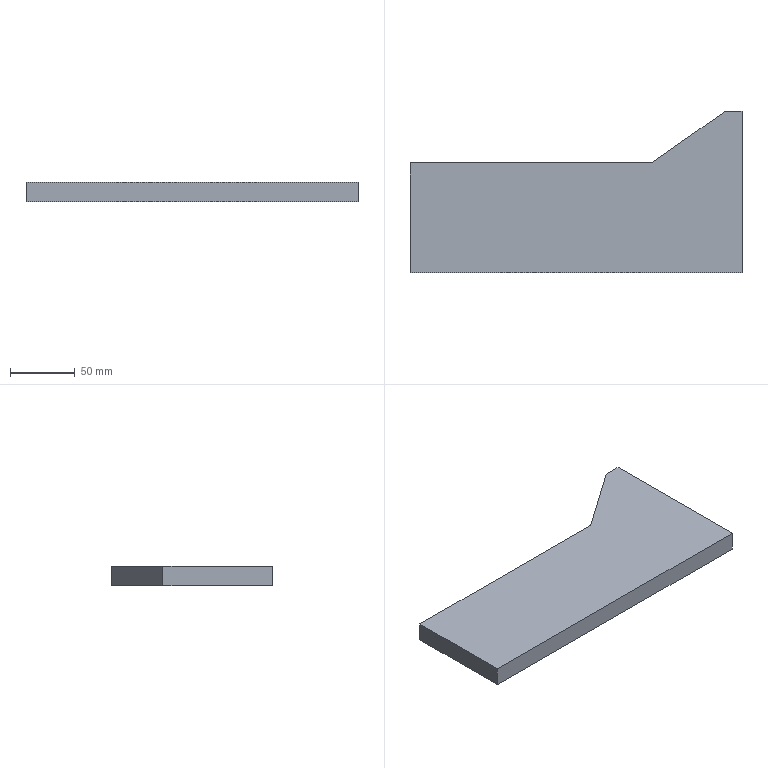Part | NX | features DATUM_CSYS 2, EXTRUDE 1, SKETCH 1 | 1 solid | 8 faces | box 257 x 125 x 15 mm | volume 352575 mm3 | plane 8
STEP:
#1=CARTESIAN_POINT('',(-257.,85.,0.));
#2=VERTEX_POINT('',#1);
#3=CARTESIAN_POINT('',(-257.,0.,0.));
#4=VERTEX_POINT('',#3);
#5=CARTESIAN_POINT('',(-257.,85.,0.));
#6=DIRECTION('',(0.,-1.,0.));
#7=VECTOR('',#6,1000.);
#8=LINE('',#5,#7);
#9=EDGE_CURVE('',#2,#4,#8,.T.);
#10=ORIENTED_EDGE('',*,*,#9,.T.);
#11=CARTESIAN_POINT('',(-257.,0.,15.));
#12=VERTEX_POINT('',#11);
#13=CARTESIAN_POINT('',(-257.,0.,15.));
#14=DIRECTION('',(0.,0.,-1.));
#15=VECTOR('',#14,1000.);
#16=LINE('',#13,#15);
#17=EDGE_CURVE('',#12,#4,#16,.T.);
#18=ORIENTED_EDGE('',*,*,#17,.F.);
#19=CARTESIAN_POINT('',(-257.,85.,15.));
#20=VERTEX_POINT('',#19);
#21=CARTESIAN_POINT('',(-257.,85.,15.));
#22=DIRECTION('',(0.,-1.,0.));
#23=VECTOR('',#22,1000.);
#24=LINE('',#21,#23);
#25=EDGE_CURVE('',#20,#12,#24,.T.);
#26=ORIENTED_EDGE('',*,*,#25,.F.);
#27=CARTESIAN_POINT('',(-257.,85.,15.));
#28=DIRECTION('',(0.,0.,-1.));
#29=VECTOR('',#28,1000.);
#30=LINE('',#27,#29);
#31=EDGE_CURVE('',#20,#2,#30,.T.);
#32=ORIENTED_EDGE('',*,*,#31,.T.);
#33=EDGE_LOOP('',(#10,#18,#26,#32));
#34=FACE_BOUND('',#33,.T.);
#35=CARTESIAN_POINT('',(-257.,85.,15.));
#36=DIRECTION('',(1.,0.,0.));
#37=DIRECTION('',(0.,1.,0.));
#38=AXIS2_PLACEMENT_3D('',#35,#36,#37);
#39=PLANE('',#38);
#40=ADVANCED_FACE('',(#34),#39,.F.);
#41=CARTESIAN_POINT('',(0.,0.,0.));
#42=VERTEX_POINT('',#41);
#43=CARTESIAN_POINT('',(-257.,0.,0.));
#44=DIRECTION('',(1.,0.,0.));
#45=VECTOR('',#44,1000.);
#46=LINE('',#43,#45);
#47=EDGE_CURVE('',#4,#42,#46,.T.);
#48=ORIENTED_EDGE('',*,*,#47,.T.);
#49=CARTESIAN_POINT('',(0.,0.,15.));
#50=VERTEX_POINT('',#49);
#51=CARTESIAN_POINT('',(0.,0.,15.));
#52=DIRECTION('',(0.,0.,-1.));
#53=VECTOR('',#52,1000.);
#54=LINE('',#51,#53);
#55=EDGE_CURVE('',#50,#42,#54,.T.);
#56=ORIENTED_EDGE('',*,*,#55,.F.);
#57=CARTESIAN_POINT('',(-257.,0.,15.));
#58=DIRECTION('',(1.,0.,0.));
#59=VECTOR('',#58,1000.);
#60=LINE('',#57,#59);
#61=EDGE_CURVE('',#12,#50,#60,.T.);
#62=ORIENTED_EDGE('',*,*,#61,.F.);
#63=ORIENTED_EDGE('',*,*,#17,.T.);
#64=EDGE_LOOP('',(#48,#56,#62,#63));
#65=FACE_BOUND('',#64,.T.);
#66=CARTESIAN_POINT('',(-257.,0.,15.));
#67=DIRECTION('',(0.,1.,0.));
#68=DIRECTION('',(-1.,0.,0.));
#69=AXIS2_PLACEMENT_3D('',#66,#67,#68);
#70=PLANE('',#69);
#71=ADVANCED_FACE('',(#65),#70,.F.);
#72=CARTESIAN_POINT('',(0.,125.,0.));
#73=VERTEX_POINT('',#72);
#74=CARTESIAN_POINT('',(0.,0.,0.));
#75=DIRECTION('',(0.,1.,0.));
#76=VECTOR('',#75,1000.);
#77=LINE('',#74,#76);
#78=EDGE_CURVE('',#42,#73,#77,.T.);
#79=ORIENTED_EDGE('',*,*,#78,.T.);
#80=CARTESIAN_POINT('',(0.,125.,15.));
#81=VERTEX_POINT('',#80);
#82=CARTESIAN_POINT('',(0.,125.,15.));
#83=DIRECTION('',(0.,0.,-1.));
#84=VECTOR('',#83,1000.);
#85=LINE('',#82,#84);
#86=EDGE_CURVE('',#81,#73,#85,.T.);
#87=ORIENTED_EDGE('',*,*,#86,.F.);
#88=CARTESIAN_POINT('',(0.,0.,15.));
#89=DIRECTION('',(0.,1.,0.));
#90=VECTOR('',#89,1000.);
#91=LINE('',#88,#90);
#92=EDGE_CURVE('',#50,#81,#91,.T.);
#93=ORIENTED_EDGE('',*,*,#92,.F.);
#94=ORIENTED_EDGE('',*,*,#55,.T.);
#95=EDGE_LOOP('',(#79,#87,#93,#94));
#96=FACE_BOUND('',#95,.T.);
#97=CARTESIAN_POINT('',(0.,0.,15.));
#98=DIRECTION('',(-1.,0.,0.));
#99=DIRECTION('',(0.,0.,1.));
#100=AXIS2_PLACEMENT_3D('',#97,#98,#99);
#101=PLANE('',#100);
#102=ADVANCED_FACE('',(#96),#101,.F.);
#103=CARTESIAN_POINT('',(-13.,125.,0.));
#104=VERTEX_POINT('',#103);
#105=CARTESIAN_POINT('',(0.,125.,0.));
#106=DIRECTION('',(-1.,0.,0.));
#107=VECTOR('',#106,1000.);
#108=LINE('',#105,#107);
#109=EDGE_CURVE('',#73,#104,#108,.T.);
#110=ORIENTED_EDGE('',*,*,#109,.T.);
#111=CARTESIAN_POINT('',(-13.,125.,15.));
#112=VERTEX_POINT('',#111);
#113=CARTESIAN_POINT('',(-13.,125.,15.));
#114=DIRECTION('',(0.,0.,-1.));
#115=VECTOR('',#114,1000.);
#116=LINE('',#113,#115);
#117=EDGE_CURVE('',#112,#104,#116,.T.);
#118=ORIENTED_EDGE('',*,*,#117,.F.);
#119=CARTESIAN_POINT('',(0.,125.,15.));
#120=DIRECTION('',(-1.,0.,0.));
#121=VECTOR('',#120,1000.);
#122=LINE('',#119,#121);
#123=EDGE_CURVE('',#81,#112,#122,.T.);
#124=ORIENTED_EDGE('',*,*,#123,.F.);
#125=ORIENTED_EDGE('',*,*,#86,.T.);
#126=EDGE_LOOP('',(#110,#118,#124,#125));
#127=FACE_BOUND('',#126,.T.);
#128=CARTESIAN_POINT('',(0.,125.,15.));
#129=DIRECTION('',(0.,-1.,0.));
#130=DIRECTION('',(1.,0.,0.));
#131=AXIS2_PLACEMENT_3D('',#128,#129,#130);
#132=PLANE('',#131);
#133=ADVANCED_FACE('',(#127),#132,.F.);
#134=CARTESIAN_POINT('',(-70.,85.,0.));
#135=VERTEX_POINT('',#134);
#136=CARTESIAN_POINT('',(-13.,125.,0.));
#137=DIRECTION('',(-0.8186,-0.5744,0.));
#138=VECTOR('',#137,1000.);
#139=LINE('',#136,#138);
#140=EDGE_CURVE('',#104,#135,#139,.T.);
#141=ORIENTED_EDGE('',*,*,#140,.T.);
#142=CARTESIAN_POINT('',(-70.,85.,15.));
#143=VERTEX_POINT('',#142);
#144=CARTESIAN_POINT('',(-70.,85.,15.));
#145=DIRECTION('',(0.,0.,-1.));
#146=VECTOR('',#145,1000.);
#147=LINE('',#144,#146);
#148=EDGE_CURVE('',#143,#135,#147,.T.);
#149=ORIENTED_EDGE('',*,*,#148,.F.);
#150=CARTESIAN_POINT('',(-13.,125.,15.));
#151=DIRECTION('',(-0.8186,-0.5744,0.));
#152=VECTOR('',#151,1000.);
#153=LINE('',#150,#152);
#154=EDGE_CURVE('',#112,#143,#153,.T.);
#155=ORIENTED_EDGE('',*,*,#154,.F.);
#156=ORIENTED_EDGE('',*,*,#117,.T.);
#157=EDGE_LOOP('',(#141,#149,#155,#156));
#158=FACE_BOUND('',#157,.T.);
#159=CARTESIAN_POINT('',(-13.,125.,15.));
#160=DIRECTION('',(0.5744,-0.8186,0.));
#161=DIRECTION('',(0.8186,0.5744,0.));
#162=AXIS2_PLACEMENT_3D('',#159,#160,#161);
#163=PLANE('',#162);
#164=ADVANCED_FACE('',(#158),#163,.F.);
#165=CARTESIAN_POINT('',(-70.,85.,0.));
#166=DIRECTION('',(-1.,0.,0.));
#167=VECTOR('',#166,1000.);
#168=LINE('',#165,#167);
#169=EDGE_CURVE('',#135,#2,#168,.T.);
#170=ORIENTED_EDGE('',*,*,#169,.T.);
#171=ORIENTED_EDGE('',*,*,#31,.F.);
#172=CARTESIAN_POINT('',(-70.,85.,15.));
#173=DIRECTION('',(-1.,0.,0.));
#174=VECTOR('',#173,1000.);
#175=LINE('',#172,#174);
#176=EDGE_CURVE('',#143,#20,#175,.T.);
#177=ORIENTED_EDGE('',*,*,#176,.F.);
#178=ORIENTED_EDGE('',*,*,#148,.T.);
#179=EDGE_LOOP('',(#170,#171,#177,#178));
#180=FACE_BOUND('',#179,.T.);
#181=CARTESIAN_POINT('',(-70.,85.,15.));
#182=DIRECTION('',(0.,-1.,0.));
#183=DIRECTION('',(1.,0.,0.));
#184=AXIS2_PLACEMENT_3D('',#181,#182,#183);
#185=PLANE('',#184);
#186=ADVANCED_FACE('',(#180),#185,.F.);
#187=ORIENTED_EDGE('',*,*,#25,.T.);
#188=ORIENTED_EDGE('',*,*,#61,.T.);
#189=ORIENTED_EDGE('',*,*,#92,.T.);
#190=ORIENTED_EDGE('',*,*,#123,.T.);
#191=ORIENTED_EDGE('',*,*,#154,.T.);
#192=ORIENTED_EDGE('',*,*,#176,.T.);
#193=EDGE_LOOP('',(#187,#188,#189,#190,#191,#192));
#194=FACE_BOUND('',#193,.T.);
#195=CARTESIAN_POINT('',(0.,0.,15.));
#196=DIRECTION('',(0.,0.,1.));
#197=DIRECTION('',(1.,0.,0.));
#198=AXIS2_PLACEMENT_3D('',#195,#196,#197);
#199=PLANE('',#198);
#200=ADVANCED_FACE('',(#194),#199,.T.);
#201=ORIENTED_EDGE('',*,*,#9,.F.);
#202=ORIENTED_EDGE('',*,*,#169,.F.);
#203=ORIENTED_EDGE('',*,*,#140,.F.);
#204=ORIENTED_EDGE('',*,*,#109,.F.);
#205=ORIENTED_EDGE('',*,*,#78,.F.);
#206=ORIENTED_EDGE('',*,*,#47,.F.);
#207=EDGE_LOOP('',(#201,#202,#203,#204,#205,#206));
#208=FACE_BOUND('',#207,.T.);
#209=CARTESIAN_POINT('',(0.,0.,0.));
#210=DIRECTION('',(0.,0.,1.));
#211=DIRECTION('',(1.,0.,0.));
#212=AXIS2_PLACEMENT_3D('',#209,#210,#211);
#213=PLANE('',#212);
#214=ADVANCED_FACE('',(#208),#213,.F.);
#215=CLOSED_SHELL('',(#40,#71,#102,#133,#164,#186,#200,#214));
#216=MANIFOLD_SOLID_BREP('',#215);
#217=(LENGTH_UNIT()NAMED_UNIT(*)SI_UNIT(.MILLI.,.METRE.));
#218=UNCERTAINTY_MEASURE_WITH_UNIT(LENGTH_MEASURE(0.00001),#217,'','');
#219=(NAMED_UNIT(*)PLANE_ANGLE_UNIT()SI_UNIT($,.RADIAN.));
#220=(NAMED_UNIT(*)SI_UNIT($,.STERADIAN.)SOLID_ANGLE_UNIT());
#221=(GEOMETRIC_REPRESENTATION_CONTEXT(3)GLOBAL_UNCERTAINTY_ASSIGNED_CONTEXT((#218))GLOBAL_UNIT_ASSIGNED_CONTEXT((#217,#219,#220))REPRESENTATION_CONTEXT('',''));
#222=ADVANCED_BREP_SHAPE_REPRESENTATION('',(#216),#221);